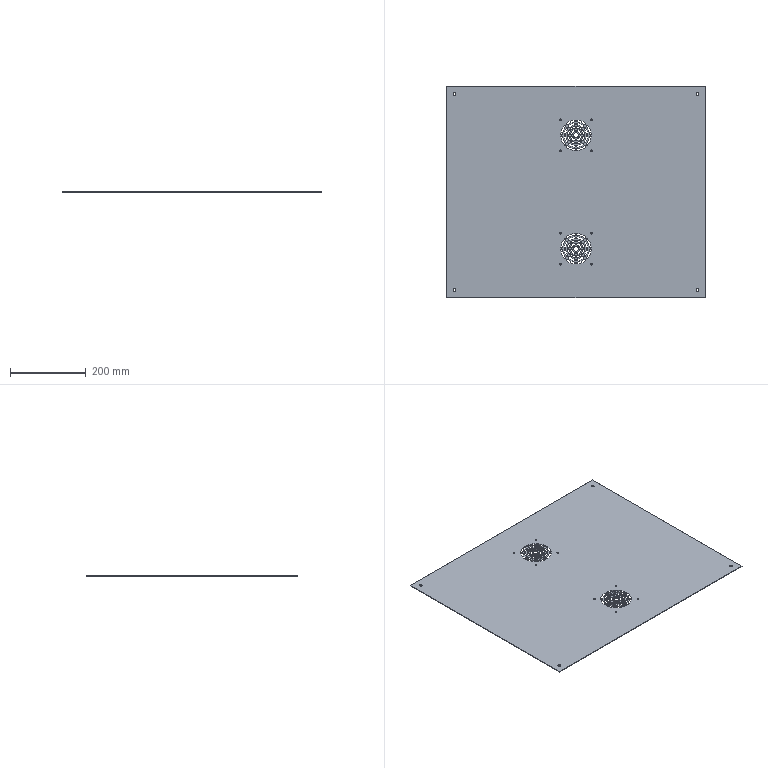Part | STEP file | 09-17 closing plate A (Default) | 1 solid | 314 faces | box 683 x 558 x 1.5 mm | volume 563276 mm3 | cylinder 308 | plane 6 | commonest cylinder face diameters 5 x168 4.5 x16 37 x16 47 x16 54 x16 64 x16